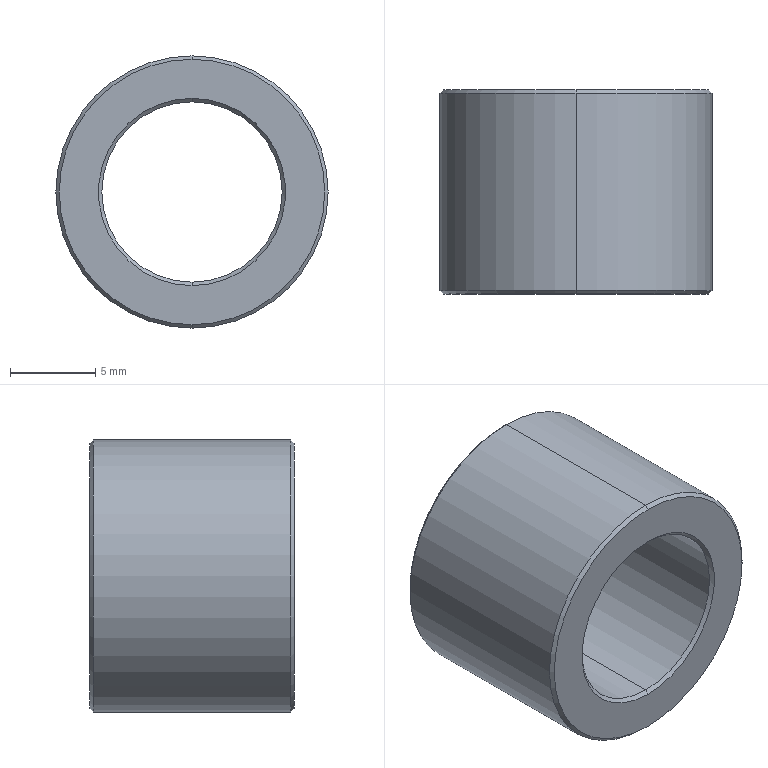Part | SolidWorks | features Chamfer 1, Extrusion 1 | 1 solid | 14 faces | box 16 x 12 x 16 mm | volume 1350 mm3 | cone 8 | cylinder 4 | plane 2 | commonest cylinder face diameters 10.6 x2 16 x2
STEP:
#1=CARTESIAN_POINT('',(0.,11.8,-5.3));
#2=VERTEX_POINT('',#1);
#3=CARTESIAN_POINT('',(0.,11.8,5.3));
#4=VERTEX_POINT('',#3);
#5=CARTESIAN_POINT('',(0.,11.8,0.));
#6=DIRECTION('',(0.,1.,0.));
#7=DIRECTION('',(0.,0.,1.));
#8=AXIS2_PLACEMENT_3D('',#5,#6,#7);
#9=CIRCLE('',#8,5.3);
#10=EDGE_CURVE('',#2,#4,#9,.T.);
#11=ORIENTED_EDGE('',*,*,#10,.F.);
#12=CARTESIAN_POINT('',(0.,12.,-5.5));
#13=VERTEX_POINT('',#12);
#14=CARTESIAN_POINT('',(0.,11.8,-5.3));
#15=DIRECTION('',(0.,0.7071,-0.7071));
#16=VECTOR('',#15,1000.);
#17=LINE('',#14,#16);
#18=EDGE_CURVE('',#2,#13,#17,.T.);
#19=ORIENTED_EDGE('',*,*,#18,.T.);
#20=CARTESIAN_POINT('',(0.,12.,5.5));
#21=VERTEX_POINT('',#20);
#22=CARTESIAN_POINT('',(0.,12.,0.));
#23=DIRECTION('',(0.,-1.,0.));
#24=DIRECTION('',(0.,0.,1.));
#25=AXIS2_PLACEMENT_3D('',#22,#23,#24);
#26=CIRCLE('',#25,5.5);
#27=EDGE_CURVE('',#21,#13,#26,.T.);
#28=ORIENTED_EDGE('',*,*,#27,.F.);
#29=CARTESIAN_POINT('',(0.,11.8,5.3));
#30=DIRECTION('',(0.,0.7071,0.7071));
#31=VECTOR('',#30,1000.);
#32=LINE('',#29,#31);
#33=EDGE_CURVE('',#4,#21,#32,.T.);
#34=ORIENTED_EDGE('',*,*,#33,.F.);
#35=EDGE_LOOP('',(#11,#19,#28,#34));
#36=FACE_OUTER_BOUND('',#35,.T.);
#37=CARTESIAN_POINT('',(0.,11.8,0.));
#38=DIRECTION('',(0.,1.,0.));
#39=DIRECTION('',(0.,0.,1.));
#40=AXIS2_PLACEMENT_3D('',#37,#38,#39);
#41=CONICAL_SURFACE('',#40,5.3,0.7854);
#42=ADVANCED_FACE('',(#36),#41,.F.);
#43=CARTESIAN_POINT('',(0.,12.,7.8));
#44=VERTEX_POINT('',#43);
#45=CARTESIAN_POINT('',(0.,12.,-7.8));
#46=VERTEX_POINT('',#45);
#47=CARTESIAN_POINT('',(0.,12.,0.));
#48=DIRECTION('',(0.,1.,0.));
#49=DIRECTION('',(0.,0.,1.));
#50=AXIS2_PLACEMENT_3D('',#47,#48,#49);
#51=CIRCLE('',#50,7.8);
#52=EDGE_CURVE('',#44,#46,#51,.T.);
#53=ORIENTED_EDGE('',*,*,#52,.F.);
#54=CARTESIAN_POINT('',(0.,11.8,8.));
#55=VERTEX_POINT('',#54);
#56=CARTESIAN_POINT('',(0.,12.,7.8));
#57=DIRECTION('',(0.,-0.7071,0.7071));
#58=VECTOR('',#57,1000.);
#59=LINE('',#56,#58);
#60=EDGE_CURVE('',#44,#55,#59,.T.);
#61=ORIENTED_EDGE('',*,*,#60,.T.);
#62=CARTESIAN_POINT('',(0.,11.8,-8.));
#63=VERTEX_POINT('',#62);
#64=CARTESIAN_POINT('',(0.,11.8,0.));
#65=DIRECTION('',(0.,-1.,0.));
#66=DIRECTION('',(0.,0.,1.));
#67=AXIS2_PLACEMENT_3D('',#64,#65,#66);
#68=CIRCLE('',#67,8.);
#69=EDGE_CURVE('',#63,#55,#68,.T.);
#70=ORIENTED_EDGE('',*,*,#69,.F.);
#71=CARTESIAN_POINT('',(0.,12.,-7.8));
#72=DIRECTION('',(0.,-0.7071,-0.7071));
#73=VECTOR('',#72,1000.);
#74=LINE('',#71,#73);
#75=EDGE_CURVE('',#46,#63,#74,.T.);
#76=ORIENTED_EDGE('',*,*,#75,.F.);
#77=EDGE_LOOP('',(#53,#61,#70,#76));
#78=FACE_OUTER_BOUND('',#77,.T.);
#79=CARTESIAN_POINT('',(0.,12.,0.));
#80=DIRECTION('',(0.,-1.,0.));
#81=DIRECTION('',(0.,0.,-1.));
#82=AXIS2_PLACEMENT_3D('',#79,#80,#81);
#83=CONICAL_SURFACE('',#82,7.8,0.7854);
#84=ADVANCED_FACE('',(#78),#83,.T.);
#85=CARTESIAN_POINT('',(0.,0.,-7.8));
#86=VERTEX_POINT('',#85);
#87=CARTESIAN_POINT('',(0.,0.,7.8));
#88=VERTEX_POINT('',#87);
#89=CARTESIAN_POINT('',(0.,0.,0.));
#90=DIRECTION('',(0.,-1.,0.));
#91=DIRECTION('',(0.,0.,1.));
#92=AXIS2_PLACEMENT_3D('',#89,#90,#91);
#93=CIRCLE('',#92,7.8);
#94=EDGE_CURVE('',#86,#88,#93,.T.);
#95=ORIENTED_EDGE('',*,*,#94,.F.);
#96=CARTESIAN_POINT('',(0.,0.2,-8.));
#97=VERTEX_POINT('',#96);
#98=CARTESIAN_POINT('',(0.,0.2,-8.));
#99=DIRECTION('',(0.,0.7071,-0.7071));
#100=VECTOR('',#99,1000.);
#101=LINE('',#98,#100);
#102=EDGE_CURVE('',#86,#97,#101,.T.);
#103=ORIENTED_EDGE('',*,*,#102,.T.);
#104=CARTESIAN_POINT('',(0.,0.2,8.));
#105=VERTEX_POINT('',#104);
#106=CARTESIAN_POINT('',(0.,0.2,0.));
#107=DIRECTION('',(0.,1.,0.));
#108=DIRECTION('',(0.,0.,1.));
#109=AXIS2_PLACEMENT_3D('',#106,#107,#108);
#110=CIRCLE('',#109,8.);
#111=EDGE_CURVE('',#105,#97,#110,.T.);
#112=ORIENTED_EDGE('',*,*,#111,.F.);
#113=CARTESIAN_POINT('',(0.,0.2,8.));
#114=DIRECTION('',(0.,0.7071,0.7071));
#115=VECTOR('',#114,1000.);
#116=LINE('',#113,#115);
#117=EDGE_CURVE('',#88,#105,#116,.T.);
#118=ORIENTED_EDGE('',*,*,#117,.F.);
#119=EDGE_LOOP('',(#95,#103,#112,#118));
#120=FACE_OUTER_BOUND('',#119,.T.);
#121=CARTESIAN_POINT('',(0.,0.2,0.));
#122=DIRECTION('',(0.,1.,0.));
#123=DIRECTION('',(0.,0.,1.));
#124=AXIS2_PLACEMENT_3D('',#121,#122,#123);
#125=CONICAL_SURFACE('',#124,8.,0.7854);
#126=ADVANCED_FACE('',(#120),#125,.T.);
#127=CARTESIAN_POINT('',(0.,0.2,5.3));
#128=VERTEX_POINT('',#127);
#129=CARTESIAN_POINT('',(0.,0.2,-5.3));
#130=VERTEX_POINT('',#129);
#131=CARTESIAN_POINT('',(0.,0.2,0.));
#132=DIRECTION('',(0.,-1.,0.));
#133=DIRECTION('',(0.,0.,1.));
#134=AXIS2_PLACEMENT_3D('',#131,#132,#133);
#135=CIRCLE('',#134,5.3);
#136=EDGE_CURVE('',#128,#130,#135,.T.);
#137=ORIENTED_EDGE('',*,*,#136,.F.);
#138=CARTESIAN_POINT('',(0.,0.,5.5));
#139=VERTEX_POINT('',#138);
#140=CARTESIAN_POINT('',(0.,0.,5.5));
#141=DIRECTION('',(0.,-0.7071,0.7071));
#142=VECTOR('',#141,1000.);
#143=LINE('',#140,#142);
#144=EDGE_CURVE('',#128,#139,#143,.T.);
#145=ORIENTED_EDGE('',*,*,#144,.T.);
#146=CARTESIAN_POINT('',(0.,0.,-5.5));
#147=VERTEX_POINT('',#146);
#148=CARTESIAN_POINT('',(0.,0.,0.));
#149=DIRECTION('',(0.,1.,0.));
#150=DIRECTION('',(0.,0.,1.));
#151=AXIS2_PLACEMENT_3D('',#148,#149,#150);
#152=CIRCLE('',#151,5.5);
#153=EDGE_CURVE('',#147,#139,#152,.T.);
#154=ORIENTED_EDGE('',*,*,#153,.F.);
#155=CARTESIAN_POINT('',(0.,0.,-5.5));
#156=DIRECTION('',(0.,-0.7071,-0.7071));
#157=VECTOR('',#156,1000.);
#158=LINE('',#155,#157);
#159=EDGE_CURVE('',#130,#147,#158,.T.);
#160=ORIENTED_EDGE('',*,*,#159,.F.);
#161=EDGE_LOOP('',(#137,#145,#154,#160));
#162=FACE_OUTER_BOUND('',#161,.T.);
#163=CARTESIAN_POINT('',(0.,0.,0.));
#164=DIRECTION('',(0.,-1.,0.));
#165=DIRECTION('',(0.,0.,-1.));
#166=AXIS2_PLACEMENT_3D('',#163,#164,#165);
#167=CONICAL_SURFACE('',#166,5.5,0.7854);
#168=ADVANCED_FACE('',(#162),#167,.F.);
#169=ORIENTED_EDGE('',*,*,#10,.T.);
#170=CARTESIAN_POINT('',(0.,12.,5.3));
#171=DIRECTION('',(0.,-1.,0.));
#172=VECTOR('',#171,1000.);
#173=LINE('',#170,#172);
#174=EDGE_CURVE('',#4,#128,#173,.T.);
#175=ORIENTED_EDGE('',*,*,#174,.T.);
#176=ORIENTED_EDGE('',*,*,#136,.T.);
#177=CARTESIAN_POINT('',(0.,12.,-5.3));
#178=DIRECTION('',(0.,-1.,0.));
#179=VECTOR('',#178,1000.);
#180=LINE('',#177,#179);
#181=EDGE_CURVE('',#2,#130,#180,.T.);
#182=ORIENTED_EDGE('',*,*,#181,.F.);
#183=EDGE_LOOP('',(#169,#175,#176,#182));
#184=FACE_OUTER_BOUND('',#183,.T.);
#185=CARTESIAN_POINT('',(0.,12.,0.));
#186=DIRECTION('',(0.,-1.,0.));
#187=DIRECTION('',(0.,0.,-1.));
#188=AXIS2_PLACEMENT_3D('',#185,#186,#187);
#189=CYLINDRICAL_SURFACE('',#188,5.3);
#190=ADVANCED_FACE('',(#184),#189,.F.);
#191=ORIENTED_EDGE('',*,*,#69,.T.);
#192=CARTESIAN_POINT('',(0.,12.,8.));
#193=DIRECTION('',(0.,-1.,0.));
#194=VECTOR('',#193,1000.);
#195=LINE('',#192,#194);
#196=EDGE_CURVE('',#55,#105,#195,.T.);
#197=ORIENTED_EDGE('',*,*,#196,.T.);
#198=ORIENTED_EDGE('',*,*,#111,.T.);
#199=CARTESIAN_POINT('',(0.,12.,-8.));
#200=DIRECTION('',(0.,-1.,0.));
#201=VECTOR('',#200,1000.);
#202=LINE('',#199,#201);
#203=EDGE_CURVE('',#63,#97,#202,.T.);
#204=ORIENTED_EDGE('',*,*,#203,.F.);
#205=EDGE_LOOP('',(#191,#197,#198,#204));
#206=FACE_OUTER_BOUND('',#205,.T.);
#207=CARTESIAN_POINT('',(0.,12.,0.));
#208=DIRECTION('',(0.,-1.,0.));
#209=DIRECTION('',(0.,0.,-1.));
#210=AXIS2_PLACEMENT_3D('',#207,#208,#209);
#211=CYLINDRICAL_SURFACE('',#210,8.);
#212=ADVANCED_FACE('',(#206),#211,.T.);
#213=CARTESIAN_POINT('',(0.,12.,0.));
#214=DIRECTION('',(0.,1.,0.));
#215=DIRECTION('',(0.,0.,1.));
#216=AXIS2_PLACEMENT_3D('',#213,#214,#215);
#217=CIRCLE('',#216,7.8);
#218=EDGE_CURVE('',#46,#44,#217,.T.);
#219=ORIENTED_EDGE('',*,*,#218,.T.);
#220=ORIENTED_EDGE('',*,*,#52,.T.);
#221=EDGE_LOOP('',(#219,#220));
#222=FACE_OUTER_BOUND('',#221,.T.);
#223=ORIENTED_EDGE('',*,*,#27,.T.);
#224=CARTESIAN_POINT('',(0.,12.,0.));
#225=DIRECTION('',(0.,-1.,0.));
#226=DIRECTION('',(0.,0.,1.));
#227=AXIS2_PLACEMENT_3D('',#224,#225,#226);
#228=CIRCLE('',#227,5.5);
#229=EDGE_CURVE('',#13,#21,#228,.T.);
#230=ORIENTED_EDGE('',*,*,#229,.T.);
#231=EDGE_LOOP('',(#223,#230));
#232=FACE_BOUND('',#231,.T.);
#233=CARTESIAN_POINT('',(0.,12.,0.));
#234=DIRECTION('',(0.,1.,0.));
#235=DIRECTION('',(0.,0.,1.));
#236=AXIS2_PLACEMENT_3D('',#233,#234,#235);
#237=PLANE('',#236);
#238=ADVANCED_FACE('',(#222,#232),#237,.T.);
#239=ORIENTED_EDGE('',*,*,#153,.T.);
#240=CARTESIAN_POINT('',(0.,0.,0.));
#241=DIRECTION('',(0.,1.,0.));
#242=DIRECTION('',(0.,0.,1.));
#243=AXIS2_PLACEMENT_3D('',#240,#241,#242);
#244=CIRCLE('',#243,5.5);
#245=EDGE_CURVE('',#139,#147,#244,.T.);
#246=ORIENTED_EDGE('',*,*,#245,.T.);
#247=EDGE_LOOP('',(#239,#246));
#248=FACE_BOUND('',#247,.T.);
#249=CARTESIAN_POINT('',(0.,0.,0.));
#250=DIRECTION('',(0.,-1.,0.));
#251=DIRECTION('',(0.,0.,1.));
#252=AXIS2_PLACEMENT_3D('',#249,#250,#251);
#253=CIRCLE('',#252,7.8);
#254=EDGE_CURVE('',#88,#86,#253,.T.);
#255=ORIENTED_EDGE('',*,*,#254,.T.);
#256=ORIENTED_EDGE('',*,*,#94,.T.);
#257=EDGE_LOOP('',(#255,#256));
#258=FACE_OUTER_BOUND('',#257,.T.);
#259=CARTESIAN_POINT('',(0.,0.,0.));
#260=DIRECTION('',(0.,1.,0.));
#261=DIRECTION('',(0.,0.,1.));
#262=AXIS2_PLACEMENT_3D('',#259,#260,#261);
#263=PLANE('',#262);
#264=ADVANCED_FACE('',(#248,#258),#263,.F.);
#265=ORIENTED_EDGE('',*,*,#196,.F.);
#266=CARTESIAN_POINT('',(0.,11.8,0.));
#267=DIRECTION('',(0.,-1.,0.));
#268=DIRECTION('',(0.,0.,1.));
#269=AXIS2_PLACEMENT_3D('',#266,#267,#268);
#270=CIRCLE('',#269,8.);
#271=EDGE_CURVE('',#55,#63,#270,.T.);
#272=ORIENTED_EDGE('',*,*,#271,.T.);
#273=ORIENTED_EDGE('',*,*,#203,.T.);
#274=CARTESIAN_POINT('',(0.,0.2,0.));
#275=DIRECTION('',(0.,1.,0.));
#276=DIRECTION('',(0.,0.,1.));
#277=AXIS2_PLACEMENT_3D('',#274,#275,#276);
#278=CIRCLE('',#277,8.);
#279=EDGE_CURVE('',#97,#105,#278,.T.);
#280=ORIENTED_EDGE('',*,*,#279,.T.);
#281=EDGE_LOOP('',(#265,#272,#273,#280));
#282=FACE_OUTER_BOUND('',#281,.T.);
#283=CARTESIAN_POINT('',(0.,12.,0.));
#284=DIRECTION('',(0.,-1.,0.));
#285=DIRECTION('',(0.,0.,-1.));
#286=AXIS2_PLACEMENT_3D('',#283,#284,#285);
#287=CYLINDRICAL_SURFACE('',#286,8.);
#288=ADVANCED_FACE('',(#282),#287,.T.);
#289=ORIENTED_EDGE('',*,*,#174,.F.);
#290=CARTESIAN_POINT('',(0.,11.8,0.));
#291=DIRECTION('',(0.,1.,0.));
#292=DIRECTION('',(0.,0.,1.));
#293=AXIS2_PLACEMENT_3D('',#290,#291,#292);
#294=CIRCLE('',#293,5.3);
#295=EDGE_CURVE('',#4,#2,#294,.T.);
#296=ORIENTED_EDGE('',*,*,#295,.T.);
#297=ORIENTED_EDGE('',*,*,#181,.T.);
#298=CARTESIAN_POINT('',(0.,0.2,0.));
#299=DIRECTION('',(0.,-1.,0.));
#300=DIRECTION('',(0.,0.,1.));
#301=AXIS2_PLACEMENT_3D('',#298,#299,#300);
#302=CIRCLE('',#301,5.3);
#303=EDGE_CURVE('',#130,#128,#302,.T.);
#304=ORIENTED_EDGE('',*,*,#303,.T.);
#305=EDGE_LOOP('',(#289,#296,#297,#304));
#306=FACE_OUTER_BOUND('',#305,.T.);
#307=CARTESIAN_POINT('',(0.,12.,0.));
#308=DIRECTION('',(0.,-1.,0.));
#309=DIRECTION('',(0.,0.,-1.));
#310=AXIS2_PLACEMENT_3D('',#307,#308,#309);
#311=CYLINDRICAL_SURFACE('',#310,5.3);
#312=ADVANCED_FACE('',(#306),#311,.F.);
#313=ORIENTED_EDGE('',*,*,#144,.F.);
#314=ORIENTED_EDGE('',*,*,#303,.F.);
#315=ORIENTED_EDGE('',*,*,#159,.T.);
#316=ORIENTED_EDGE('',*,*,#245,.F.);
#317=EDGE_LOOP('',(#313,#314,#315,#316));
#318=FACE_OUTER_BOUND('',#317,.T.);
#319=CARTESIAN_POINT('',(0.,0.,0.));
#320=DIRECTION('',(0.,-1.,0.));
#321=DIRECTION('',(0.,0.,-1.));
#322=AXIS2_PLACEMENT_3D('',#319,#320,#321);
#323=CONICAL_SURFACE('',#322,5.5,0.7854);
#324=ADVANCED_FACE('',(#318),#323,.F.);
#325=ORIENTED_EDGE('',*,*,#102,.F.);
#326=ORIENTED_EDGE('',*,*,#254,.F.);
#327=ORIENTED_EDGE('',*,*,#117,.T.);
#328=ORIENTED_EDGE('',*,*,#279,.F.);
#329=EDGE_LOOP('',(#325,#326,#327,#328));
#330=FACE_OUTER_BOUND('',#329,.T.);
#331=CARTESIAN_POINT('',(0.,0.2,0.));
#332=DIRECTION('',(0.,1.,0.));
#333=DIRECTION('',(0.,0.,1.));
#334=AXIS2_PLACEMENT_3D('',#331,#332,#333);
#335=CONICAL_SURFACE('',#334,8.,0.7854);
#336=ADVANCED_FACE('',(#330),#335,.T.);
#337=ORIENTED_EDGE('',*,*,#60,.F.);
#338=ORIENTED_EDGE('',*,*,#218,.F.);
#339=ORIENTED_EDGE('',*,*,#75,.T.);
#340=ORIENTED_EDGE('',*,*,#271,.F.);
#341=EDGE_LOOP('',(#337,#338,#339,#340));
#342=FACE_OUTER_BOUND('',#341,.T.);
#343=CARTESIAN_POINT('',(0.,12.,0.));
#344=DIRECTION('',(0.,-1.,0.));
#345=DIRECTION('',(0.,0.,-1.));
#346=AXIS2_PLACEMENT_3D('',#343,#344,#345);
#347=CONICAL_SURFACE('',#346,7.8,0.7854);
#348=ADVANCED_FACE('',(#342),#347,.T.);
#349=ORIENTED_EDGE('',*,*,#18,.F.);
#350=ORIENTED_EDGE('',*,*,#295,.F.);
#351=ORIENTED_EDGE('',*,*,#33,.T.);
#352=ORIENTED_EDGE('',*,*,#229,.F.);
#353=EDGE_LOOP('',(#349,#350,#351,#352));
#354=FACE_OUTER_BOUND('',#353,.T.);
#355=CARTESIAN_POINT('',(0.,11.8,0.));
#356=DIRECTION('',(0.,1.,0.));
#357=DIRECTION('',(0.,0.,1.));
#358=AXIS2_PLACEMENT_3D('',#355,#356,#357);
#359=CONICAL_SURFACE('',#358,5.3,0.7854);
#360=ADVANCED_FACE('',(#354),#359,.F.);
#361=CLOSED_SHELL('',(#42,#84,#126,#168,#190,#212,#238,#264,#288,#312,#324,#336,#348,#360));
#362=MANIFOLD_SOLID_BREP('',#361);
#363=CARTESIAN_POINT('',(0.,0.,0.));
#364=DIRECTION('',(0.,0.,1.));
#365=DIRECTION('',(1.,0.,0.));
#366=AXIS2_PLACEMENT_3D('',#363,#364,#365);
#367=(LENGTH_UNIT()NAMED_UNIT(*)SI_UNIT(.MILLI.,.METRE.));
#368=UNCERTAINTY_MEASURE_WITH_UNIT(LENGTH_MEASURE(0.00001),#367,'','');
#369=(NAMED_UNIT(*)PLANE_ANGLE_UNIT()SI_UNIT($,.RADIAN.));
#370=(NAMED_UNIT(*)SI_UNIT($,.STERADIAN.)SOLID_ANGLE_UNIT());
#371=(GEOMETRIC_REPRESENTATION_CONTEXT(3)GLOBAL_UNCERTAINTY_ASSIGNED_CONTEXT((#368))GLOBAL_UNIT_ASSIGNED_CONTEXT((#367,#369,#370))REPRESENTATION_CONTEXT('',''));
#372=ADVANCED_BREP_SHAPE_REPRESENTATION('',(#362,#366),#371);